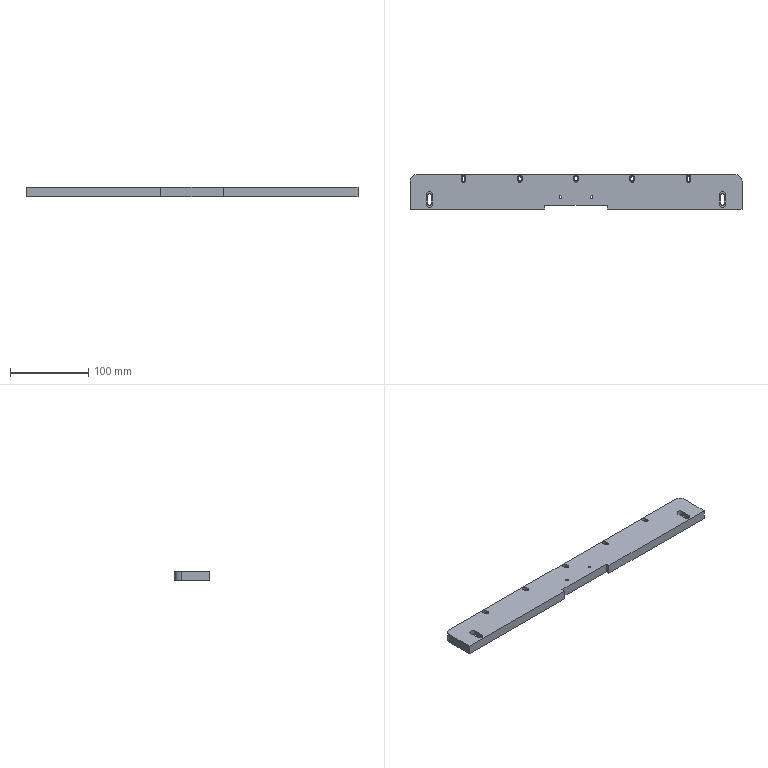Part | SolidWorks | features ICE 6, Extrusion 1, Fillet 1, HoleWzd 1, LPattern 1 | 1 solid | 99 faces | box 425 x 44 x 12 mm | volume 214700 mm3 | plane 65 | cylinder 34 | commonest cylinder face diameters 3.2 x10 6 x10 3.3 x4 4 x4 8 x4 16 x2